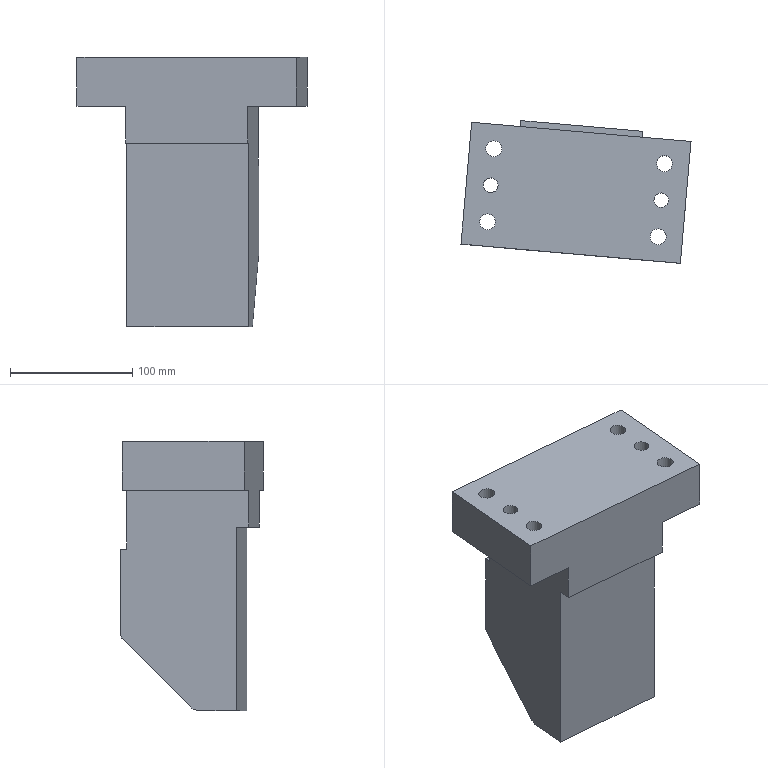Part | NX | features solid 2 | 1 solid | 33 faces | box 188.031 x 116.802 x 220 mm | volume 2209901 mm3 | plane 18 | cylinder 11 | spline 3 | cone 1 | commonest cylinder face diameters 13 x4 20 x4 12 x3
STEP:
#1=CARTESIAN_POINT('',(273.786,-317.22,-120.));
#2=VERTEX_POINT('',#1);
#3=CARTESIAN_POINT('',(273.786,-311.22,-120.));
#4=DIRECTION('',(0.,0.,1.));
#5=DIRECTION('',(0.,-1.,0.));
#6=AXIS2_PLACEMENT_3D('',#3,#4,#5);
#7=CIRCLE('',#6,6.);
#8=EDGE_CURVE('',#2,#2,#7,.T.);
#9=ORIENTED_EDGE('',*,*,#8,.T.);
#10=EDGE_LOOP('',(#9));
#11=FACE_BOUND('',#10,.T.);
#12=CARTESIAN_POINT('',(225.156,-294.888,-120.));
#13=VERTEX_POINT('',#12);
#14=CARTESIAN_POINT('',(222.466,-325.628,-120.));
#15=VERTEX_POINT('',#14);
#16=CARTESIAN_POINT('',(230.746,-230.99,-120.));
#17=DIRECTION('',(-0.08716,-0.9962,0.));
#18=VECTOR('',#17,1000.);
#19=LINE('',#16,#18);
#20=EDGE_CURVE('',#13,#15,#19,.T.);
#21=ORIENTED_EDGE('',*,*,#20,.F.);
#22=CARTESIAN_POINT('',(324.775,-303.603,-120.));
#23=VERTEX_POINT('',#22);
#24=CARTESIAN_POINT('',(225.156,-294.888,-120.));
#25=CARTESIAN_POINT('',(258.362,-297.793,-120.));
#26=CARTESIAN_POINT('',(291.569,-300.698,-120.));
#27=CARTESIAN_POINT('',(324.775,-303.603,-120.));
#28=B_SPLINE_CURVE_WITH_KNOTS('',3,(#24,#25,#26,#27),.UNSPECIFIED.,.F.,.F.,(4,4),(0.,0.1),.UNSPECIFIED.);
#29=EDGE_CURVE('',#13,#23,#28,.T.);
#30=ORIENTED_EDGE('',*,*,#29,.T.);
#31=CARTESIAN_POINT('',(322.086,-334.344,-120.));
#32=VERTEX_POINT('',#31);
#33=CARTESIAN_POINT('',(330.365,-239.705,-120.));
#34=DIRECTION('',(-0.08716,-0.9962,0.));
#35=VECTOR('',#34,1000.);
#36=LINE('',#33,#35);
#37=EDGE_CURVE('',#23,#32,#36,.T.);
#38=ORIENTED_EDGE('',*,*,#37,.T.);
#39=CARTESIAN_POINT('',(322.086,-334.344,-120.));
#40=DIRECTION('',(0.9962,-0.08716,0.));
#41=VECTOR('',#40,1000.);
#42=LINE('',#39,#41);
#43=EDGE_CURVE('',#15,#32,#42,.T.);
#44=ORIENTED_EDGE('',*,*,#43,.F.);
#45=EDGE_LOOP('',(#21,#30,#38,#44));
#46=FACE_BOUND('',#45,.T.);
#47=CARTESIAN_POINT('',(330.365,-239.705,-120.));
#48=DIRECTION('',(0.,0.,-1.));
#49=DIRECTION('',(0.,1.,0.));
#50=AXIS2_PLACEMENT_3D('',#47,#48,#49);
#51=PLANE('',#50);
#52=ADVANCED_FACE('',(#11,#46),#51,.T.);
#53=CARTESIAN_POINT('',(230.618,-232.449,-61.464));
#54=VERTEX_POINT('',#53);
#55=CARTESIAN_POINT('',(225.772,-287.844,-117.071));
#56=VERTEX_POINT('',#55);
#57=CARTESIAN_POINT('',(228.872,-252.408,-81.5));
#58=DIRECTION('',(-0.06163,-0.7044,-0.7071));
#59=VECTOR('',#58,1000.);
#60=LINE('',#57,#59);
#61=EDGE_CURVE('',#54,#56,#60,.T.);
#62=ORIENTED_EDGE('',*,*,#61,.T.);
#63=CARTESIAN_POINT('',(225.156,-294.888,-110.));
#64=DIRECTION('',(-0.9962,0.08716,0.));
#65=DIRECTION('',(-0.08716,-0.9962,0.));
#66=AXIS2_PLACEMENT_3D('',#63,#64,#65);
#67=CIRCLE('',#66,10.);
#68=EDGE_CURVE('',#56,#13,#67,.T.);
#69=ORIENTED_EDGE('',*,*,#68,.T.);
#70=ORIENTED_EDGE('',*,*,#20,.T.);
#71=CARTESIAN_POINT('',(222.466,-325.628,30.));
#72=VERTEX_POINT('',#71);
#73=CARTESIAN_POINT('',(222.466,-325.628,-170.));
#74=DIRECTION('',(0.,0.,1.));
#75=VECTOR('',#74,1000.);
#76=LINE('',#73,#75);
#77=EDGE_CURVE('',#72,#15,#76,.F.);
#78=ORIENTED_EDGE('',*,*,#77,.F.);
#79=CARTESIAN_POINT('',(221.595,-335.59,30.));
#80=VERTEX_POINT('',#79);
#81=CARTESIAN_POINT('',(220.723,-345.552,30.));
#82=DIRECTION('',(-0.08716,-0.9962,0.));
#83=VECTOR('',#82,1000.);
#84=LINE('',#81,#83);
#85=EDGE_CURVE('',#80,#72,#84,.F.);
#86=ORIENTED_EDGE('',*,*,#85,.F.);
#87=CARTESIAN_POINT('',(221.595,-335.59,60.));
#88=VERTEX_POINT('',#87);
#89=CARTESIAN_POINT('',(221.595,-335.59,-103.));
#90=DIRECTION('',(0.,0.,1.));
#91=VECTOR('',#90,1000.);
#92=LINE('',#89,#91);
#93=EDGE_CURVE('',#80,#88,#92,.T.);
#94=ORIENTED_EDGE('',*,*,#93,.T.);
#95=CARTESIAN_POINT('',(230.31,-235.971,60.));
#96=VERTEX_POINT('',#95);
#97=CARTESIAN_POINT('',(212.443,-440.191,60.));
#98=DIRECTION('',(0.08716,0.9962,0.));
#99=VECTOR('',#98,1000.);
#100=LINE('',#97,#99);
#101=EDGE_CURVE('',#88,#96,#100,.T.);
#102=ORIENTED_EDGE('',*,*,#101,.T.);
#103=CARTESIAN_POINT('',(230.31,-235.971,12.));
#104=VERTEX_POINT('',#103);
#105=CARTESIAN_POINT('',(230.31,-235.971,57.));
#106=DIRECTION('',(0.,0.,-1.));
#107=VECTOR('',#106,1000.);
#108=LINE('',#105,#107);
#109=EDGE_CURVE('',#96,#104,#108,.T.);
#110=ORIENTED_EDGE('',*,*,#109,.T.);
#111=CARTESIAN_POINT('',(230.746,-230.99,12.));
#112=VERTEX_POINT('',#111);
#113=CARTESIAN_POINT('',(230.746,-230.99,12.));
#114=DIRECTION('',(0.08716,0.9962,0.));
#115=VECTOR('',#114,1000.);
#116=LINE('',#113,#115);
#117=EDGE_CURVE('',#104,#112,#116,.T.);
#118=ORIENTED_EDGE('',*,*,#117,.T.);
#119=CARTESIAN_POINT('',(230.746,-230.99,-57.929));
#120=VERTEX_POINT('',#119);
#121=CARTESIAN_POINT('',(230.746,-230.99,-103.));
#122=DIRECTION('',(0.,0.,1.));
#123=VECTOR('',#122,1000.);
#124=LINE('',#121,#123);
#125=EDGE_CURVE('',#112,#120,#124,.F.);
#126=ORIENTED_EDGE('',*,*,#125,.T.);
#127=CARTESIAN_POINT('',(230.31,-235.971,-57.929));
#128=DIRECTION('',(-0.9962,0.08716,0.));
#129=DIRECTION('',(-0.08716,-0.9962,0.));
#130=AXIS2_PLACEMENT_3D('',#127,#128,#129);
#131=CIRCLE('',#130,5.);
#132=EDGE_CURVE('',#120,#54,#131,.T.);
#133=ORIENTED_EDGE('',*,*,#132,.T.);
#134=EDGE_LOOP('',(#62,#69,#70,#78,#86,#94,#102,#110,#118,#126,#133));
#135=FACE_BOUND('',#134,.T.);
#136=CARTESIAN_POINT('',(230.746,-230.99,-103.));
#137=DIRECTION('',(-0.9962,0.08716,0.));
#138=DIRECTION('',(0.,0.,1.));
#139=AXIS2_PLACEMENT_3D('',#136,#137,#138);
#140=PLANE('',#139);
#141=ADVANCED_FACE('',(#135),#140,.T.);
#142=ORIENTED_EDGE('',*,*,#37,.F.);
#143=CARTESIAN_POINT('',(325.391,-296.559,-117.071));
#144=VERTEX_POINT('',#143);
#145=CARTESIAN_POINT('',(324.775,-303.603,-110.));
#146=DIRECTION('',(-0.9962,0.08716,0.));
#147=DIRECTION('',(-0.08716,-0.9962,0.));
#148=AXIS2_PLACEMENT_3D('',#145,#146,#147);
#149=CIRCLE('',#148,10.);
#150=EDGE_CURVE('',#23,#144,#149,.F.);
#151=ORIENTED_EDGE('',*,*,#150,.T.);
#152=CARTESIAN_POINT('',(330.238,-241.164,-61.464));
#153=VERTEX_POINT('',#152);
#154=CARTESIAN_POINT('',(328.492,-261.124,-81.5));
#155=DIRECTION('',(-0.06163,-0.7044,-0.7071));
#156=VECTOR('',#155,1000.);
#157=LINE('',#154,#156);
#158=EDGE_CURVE('',#153,#144,#157,.T.);
#159=ORIENTED_EDGE('',*,*,#158,.F.);
#160=CARTESIAN_POINT('',(330.365,-239.705,-57.929));
#161=VERTEX_POINT('',#160);
#162=CARTESIAN_POINT('',(329.93,-244.686,-57.929));
#163=DIRECTION('',(-0.9962,0.08716,0.));
#164=DIRECTION('',(-0.08716,-0.9962,0.));
#165=AXIS2_PLACEMENT_3D('',#162,#163,#164);
#166=CIRCLE('',#165,5.);
#167=EDGE_CURVE('',#153,#161,#166,.F.);
#168=ORIENTED_EDGE('',*,*,#167,.T.);
#169=CARTESIAN_POINT('',(330.365,-239.705,12.));
#170=VERTEX_POINT('',#169);
#171=CARTESIAN_POINT('',(330.365,-239.705,-103.));
#172=DIRECTION('',(0.,0.,1.));
#173=VECTOR('',#172,1000.);
#174=LINE('',#171,#173);
#175=EDGE_CURVE('',#170,#161,#174,.F.);
#176=ORIENTED_EDGE('',*,*,#175,.F.);
#177=CARTESIAN_POINT('',(329.93,-244.686,12.));
#178=VERTEX_POINT('',#177);
#179=CARTESIAN_POINT('',(330.365,-239.705,12.));
#180=DIRECTION('',(0.08716,0.9962,0.));
#181=VECTOR('',#180,1000.);
#182=LINE('',#179,#181);
#183=EDGE_CURVE('',#178,#170,#182,.T.);
#184=ORIENTED_EDGE('',*,*,#183,.F.);
#185=CARTESIAN_POINT('',(329.93,-244.686,60.));
#186=VERTEX_POINT('',#185);
#187=CARTESIAN_POINT('',(329.93,-244.686,57.));
#188=DIRECTION('',(0.,0.,-1.));
#189=VECTOR('',#188,1000.);
#190=LINE('',#187,#189);
#191=EDGE_CURVE('',#186,#178,#190,.T.);
#192=ORIENTED_EDGE('',*,*,#191,.F.);
#193=CARTESIAN_POINT('',(321.214,-344.306,60.));
#194=VERTEX_POINT('',#193);
#195=CARTESIAN_POINT('',(312.063,-448.906,60.));
#196=DIRECTION('',(0.08716,0.9962,0.));
#197=VECTOR('',#196,1000.);
#198=LINE('',#195,#197);
#199=EDGE_CURVE('',#194,#186,#198,.T.);
#200=ORIENTED_EDGE('',*,*,#199,.F.);
#201=CARTESIAN_POINT('',(321.214,-344.306,30.));
#202=VERTEX_POINT('',#201);
#203=CARTESIAN_POINT('',(321.214,-344.306,-103.));
#204=DIRECTION('',(0.,0.,1.));
#205=VECTOR('',#204,1000.);
#206=LINE('',#203,#205);
#207=EDGE_CURVE('',#202,#194,#206,.T.);
#208=ORIENTED_EDGE('',*,*,#207,.F.);
#209=CARTESIAN_POINT('',(322.086,-334.344,30.));
#210=VERTEX_POINT('',#209);
#211=CARTESIAN_POINT('',(320.343,-354.268,30.));
#212=DIRECTION('',(-0.08716,-0.9962,0.));
#213=VECTOR('',#212,1000.);
#214=LINE('',#211,#213);
#215=EDGE_CURVE('',#202,#210,#214,.F.);
#216=ORIENTED_EDGE('',*,*,#215,.T.);
#217=CARTESIAN_POINT('',(322.086,-334.344,-170.));
#218=DIRECTION('',(0.,0.,-1.));
#219=VECTOR('',#218,1000.);
#220=LINE('',#217,#219);
#221=EDGE_CURVE('',#32,#210,#220,.F.);
#222=ORIENTED_EDGE('',*,*,#221,.F.);
#223=EDGE_LOOP('',(#142,#151,#159,#168,#176,#184,#192,#200,#208,#216,#222));
#224=FACE_BOUND('',#223,.T.);
#225=CARTESIAN_POINT('',(330.365,-239.705,-103.));
#226=DIRECTION('',(-0.9962,0.08716,0.));
#227=DIRECTION('',(0.,0.,1.));
#228=AXIS2_PLACEMENT_3D('',#225,#226,#227);
#229=PLANE('',#228);
#230=ADVANCED_FACE('',(#224),#229,.F.);
#231=ORIENTED_EDGE('',*,*,#175,.T.);
#232=CARTESIAN_POINT('',(330.365,-239.705,-57.929));
#233=CARTESIAN_POINT('',(297.159,-236.8,-57.929));
#234=CARTESIAN_POINT('',(263.952,-233.895,-57.929));
#235=CARTESIAN_POINT('',(230.746,-230.99,-57.929));
#236=B_SPLINE_CURVE_WITH_KNOTS('',3,(#232,#233,#234,#235),.UNSPECIFIED.,.F.,.F.,(4,4),(0.,0.1),.UNSPECIFIED.);
#237=EDGE_CURVE('',#161,#120,#236,.T.);
#238=ORIENTED_EDGE('',*,*,#237,.T.);
#239=ORIENTED_EDGE('',*,*,#125,.F.);
#240=CARTESIAN_POINT('',(330.365,-239.705,12.));
#241=DIRECTION('',(0.9962,-0.08716,0.));
#242=VECTOR('',#241,1000.);
#243=LINE('',#240,#242);
#244=EDGE_CURVE('',#170,#112,#243,.F.);
#245=ORIENTED_EDGE('',*,*,#244,.F.);
#246=EDGE_LOOP('',(#231,#238,#239,#245));
#247=FACE_BOUND('',#246,.T.);
#248=CARTESIAN_POINT('',(330.365,-239.705,-80.));
#249=DIRECTION('',(-0.08716,-0.9962,0.));
#250=DIRECTION('',(0.9962,-0.08716,0.));
#251=AXIS2_PLACEMENT_3D('',#248,#249,#250);
#252=PLANE('',#251);
#253=ADVANCED_FACE('',(#247),#252,.F.);
#254=ORIENTED_EDGE('',*,*,#93,.F.);
#255=CARTESIAN_POINT('',(321.214,-344.306,30.));
#256=DIRECTION('',(-0.9962,0.08716,0.));
#257=VECTOR('',#256,1000.);
#258=LINE('',#255,#257);
#259=EDGE_CURVE('',#80,#202,#258,.F.);
#260=ORIENTED_EDGE('',*,*,#259,.T.);
#261=ORIENTED_EDGE('',*,*,#207,.T.);
#262=CARTESIAN_POINT('',(361.062,-347.792,60.));
#263=VERTEX_POINT('',#262);
#264=CARTESIAN_POINT('',(321.214,-344.306,60.));
#265=DIRECTION('',(-0.9962,0.08716,0.));
#266=VECTOR('',#265,1000.);
#267=LINE('',#264,#266);
#268=EDGE_CURVE('',#263,#194,#267,.T.);
#269=ORIENTED_EDGE('',*,*,#268,.F.);
#270=CARTESIAN_POINT('',(361.062,-347.792,100.));
#271=VERTEX_POINT('',#270);
#272=CARTESIAN_POINT('',(361.062,-347.792,102.));
#273=DIRECTION('',(0.,0.,-1.));
#274=VECTOR('',#273,1000.);
#275=LINE('',#272,#274);
#276=EDGE_CURVE('',#271,#263,#275,.T.);
#277=ORIENTED_EDGE('',*,*,#276,.F.);
#278=CARTESIAN_POINT('',(181.747,-332.104,100.));
#279=VERTEX_POINT('',#278);
#280=CARTESIAN_POINT('',(321.214,-344.306,100.));
#281=DIRECTION('',(-0.9962,0.08716,0.));
#282=VECTOR('',#281,1000.);
#283=LINE('',#280,#282);
#284=EDGE_CURVE('',#271,#279,#283,.T.);
#285=ORIENTED_EDGE('',*,*,#284,.T.);
#286=CARTESIAN_POINT('',(181.747,-332.104,60.));
#287=VERTEX_POINT('',#286);
#288=CARTESIAN_POINT('',(181.747,-332.104,-103.));
#289=DIRECTION('',(0.,0.,-1.));
#290=VECTOR('',#289,1000.);
#291=LINE('',#288,#290);
#292=EDGE_CURVE('',#279,#287,#291,.T.);
#293=ORIENTED_EDGE('',*,*,#292,.T.);
#294=CARTESIAN_POINT('',(108.527,-325.698,60.));
#295=DIRECTION('',(0.9962,-0.08716,0.));
#296=VECTOR('',#295,1000.);
#297=LINE('',#294,#296);
#298=EDGE_CURVE('',#287,#88,#297,.T.);
#299=ORIENTED_EDGE('',*,*,#298,.T.);
#300=EDGE_LOOP('',(#254,#260,#261,#269,#277,#285,#293,#299));
#301=FACE_BOUND('',#300,.T.);
#302=CARTESIAN_POINT('',(321.214,-344.306,-103.));
#303=DIRECTION('',(-0.08716,-0.9962,0.));
#304=DIRECTION('',(0.,0.,-1.));
#305=AXIS2_PLACEMENT_3D('',#302,#303,#304);
#306=PLANE('',#305);
#307=ADVANCED_FACE('',(#301),#306,.T.);
#308=CARTESIAN_POINT('',(329.93,-244.686,12.));
#309=DIRECTION('',(-0.9962,0.08716,0.));
#310=VECTOR('',#309,1000.);
#311=LINE('',#308,#310);
#312=EDGE_CURVE('',#178,#104,#311,.T.);
#313=ORIENTED_EDGE('',*,*,#312,.F.);
#314=ORIENTED_EDGE('',*,*,#183,.T.);
#315=ORIENTED_EDGE('',*,*,#244,.T.);
#316=ORIENTED_EDGE('',*,*,#117,.F.);
#317=EDGE_LOOP('',(#313,#314,#315,#316));
#318=FACE_BOUND('',#317,.T.);
#319=CARTESIAN_POINT('',(327.751,-269.591,12.));
#320=DIRECTION('',(0.,0.,1.));
#321=DIRECTION('',(0.,-1.,0.));
#322=AXIS2_PLACEMENT_3D('',#319,#320,#321);
#323=PLANE('',#322);
#324=ADVANCED_FACE('',(#318),#323,.T.);
#325=ORIENTED_EDGE('',*,*,#312,.T.);
#326=ORIENTED_EDGE('',*,*,#109,.F.);
#327=CARTESIAN_POINT('',(190.462,-232.485,60.));
#328=VERTEX_POINT('',#327);
#329=CARTESIAN_POINT('',(117.242,-226.079,60.));
#330=DIRECTION('',(0.9962,-0.08716,0.));
#331=VECTOR('',#330,1000.);
#332=LINE('',#329,#331);
#333=EDGE_CURVE('',#328,#96,#332,.T.);
#334=ORIENTED_EDGE('',*,*,#333,.F.);
#335=CARTESIAN_POINT('',(190.462,-232.485,100.));
#336=VERTEX_POINT('',#335);
#337=CARTESIAN_POINT('',(190.462,-232.485,57.));
#338=DIRECTION('',(0.,0.,-1.));
#339=VECTOR('',#338,1000.);
#340=LINE('',#337,#339);
#341=EDGE_CURVE('',#336,#328,#340,.T.);
#342=ORIENTED_EDGE('',*,*,#341,.F.);
#343=CARTESIAN_POINT('',(369.777,-248.173,100.));
#344=VERTEX_POINT('',#343);
#345=CARTESIAN_POINT('',(329.93,-244.686,100.));
#346=DIRECTION('',(-0.9962,0.08716,0.));
#347=VECTOR('',#346,1000.);
#348=LINE('',#345,#347);
#349=EDGE_CURVE('',#344,#336,#348,.T.);
#350=ORIENTED_EDGE('',*,*,#349,.F.);
#351=CARTESIAN_POINT('',(369.777,-248.173,60.));
#352=VERTEX_POINT('',#351);
#353=CARTESIAN_POINT('',(369.777,-248.173,102.));
#354=DIRECTION('',(0.,0.,-1.));
#355=VECTOR('',#354,1000.);
#356=LINE('',#353,#355);
#357=EDGE_CURVE('',#344,#352,#356,.T.);
#358=ORIENTED_EDGE('',*,*,#357,.T.);
#359=CARTESIAN_POINT('',(267.667,-239.239,60.));
#360=DIRECTION('',(-0.9962,0.08716,0.));
#361=VECTOR('',#360,1000.);
#362=LINE('',#359,#361);
#363=EDGE_CURVE('',#352,#186,#362,.T.);
#364=ORIENTED_EDGE('',*,*,#363,.T.);
#365=ORIENTED_EDGE('',*,*,#191,.T.);
#366=EDGE_LOOP('',(#325,#326,#334,#342,#350,#358,#364,#365));
#367=FACE_BOUND('',#366,.T.);
#368=CARTESIAN_POINT('',(329.93,-244.686,57.));
#369=DIRECTION('',(-0.08716,-0.9962,0.));
#370=DIRECTION('',(0.9962,-0.08716,0.));
#371=AXIS2_PLACEMENT_3D('',#368,#369,#370);
#372=PLANE('',#371);
#373=ADVANCED_FACE('',(#367),#372,.F.);
#374=CARTESIAN_POINT('',(206.029,-290.037,100.));
#375=VERTEX_POINT('',#374);
#376=CARTESIAN_POINT('',(206.029,-284.037,100.));
#377=DIRECTION('',(0.,0.,1.));
#378=DIRECTION('',(0.,-1.,0.));
#379=AXIS2_PLACEMENT_3D('',#376,#377,#378);
#380=CIRCLE('',#379,6.);
#381=EDGE_CURVE('',#375,#375,#380,.T.);
#382=ORIENTED_EDGE('',*,*,#381,.F.);
#383=EDGE_LOOP('',(#382));
#384=FACE_BOUND('',#383,.T.);
#385=CARTESIAN_POINT('',(345.496,-302.239,100.));
#386=VERTEX_POINT('',#385);
#387=CARTESIAN_POINT('',(345.496,-296.239,100.));
#388=DIRECTION('',(0.,0.,1.));
#389=DIRECTION('',(0.,-1.,0.));
#390=AXIS2_PLACEMENT_3D('',#387,#388,#389);
#391=CIRCLE('',#390,6.);
#392=EDGE_CURVE('',#386,#386,#391,.T.);
#393=ORIENTED_EDGE('',*,*,#392,.F.);
#394=EDGE_LOOP('',(#393));
#395=FACE_BOUND('',#394,.T.);
#396=CARTESIAN_POINT('',(203.414,-320.423,100.));
#397=VERTEX_POINT('',#396);
#398=CARTESIAN_POINT('',(203.414,-313.923,100.));
#399=DIRECTION('',(0.,0.,1.));
#400=DIRECTION('',(0.,-1.,0.));
#401=AXIS2_PLACEMENT_3D('',#398,#399,#400);
#402=CIRCLE('',#401,6.5);
#403=EDGE_CURVE('',#397,#397,#402,.T.);
#404=ORIENTED_EDGE('',*,*,#403,.F.);
#405=EDGE_LOOP('',(#404));
#406=FACE_BOUND('',#405,.T.);
#407=CARTESIAN_POINT('',(208.643,-260.652,100.));
#408=VERTEX_POINT('',#407);
#409=CARTESIAN_POINT('',(208.643,-254.152,100.));
#410=DIRECTION('',(0.,0.,1.));
#411=DIRECTION('',(0.,-1.,0.));
#412=AXIS2_PLACEMENT_3D('',#409,#410,#411);
#413=CIRCLE('',#412,6.5);
#414=EDGE_CURVE('',#408,#408,#413,.T.);
#415=ORIENTED_EDGE('',*,*,#414,.F.);
#416=EDGE_LOOP('',(#415));
#417=FACE_BOUND('',#416,.T.);
#418=CARTESIAN_POINT('',(342.881,-332.625,100.));
#419=VERTEX_POINT('',#418);
#420=CARTESIAN_POINT('',(342.881,-326.125,100.));
#421=DIRECTION('',(0.,0.,1.));
#422=DIRECTION('',(0.,-1.,0.));
#423=AXIS2_PLACEMENT_3D('',#420,#421,#422);
#424=CIRCLE('',#423,6.5);
#425=EDGE_CURVE('',#419,#419,#424,.T.);
#426=ORIENTED_EDGE('',*,*,#425,.F.);
#427=EDGE_LOOP('',(#426));
#428=FACE_BOUND('',#427,.T.);
#429=CARTESIAN_POINT('',(348.11,-272.853,100.));
#430=VERTEX_POINT('',#429);
#431=CARTESIAN_POINT('',(348.11,-266.353,100.));
#432=DIRECTION('',(0.,0.,1.));
#433=DIRECTION('',(0.,-1.,0.));
#434=AXIS2_PLACEMENT_3D('',#431,#432,#433);
#435=CIRCLE('',#434,6.5);
#436=EDGE_CURVE('',#430,#430,#435,.T.);
#437=ORIENTED_EDGE('',*,*,#436,.F.);
#438=EDGE_LOOP('',(#437));
#439=FACE_BOUND('',#438,.T.);
#440=ORIENTED_EDGE('',*,*,#349,.T.);
#441=CARTESIAN_POINT('',(177.326,-382.632,100.));
#442=DIRECTION('',(0.08716,0.9962,0.));
#443=VECTOR('',#442,1000.);
#444=LINE('',#441,#443);
#445=EDGE_CURVE('',#279,#336,#444,.T.);
#446=ORIENTED_EDGE('',*,*,#445,.F.);
#447=ORIENTED_EDGE('',*,*,#284,.F.);
#448=CARTESIAN_POINT('',(367.599,-273.077,100.));
#449=DIRECTION('',(0.08716,0.9962,0.));
#450=VECTOR('',#449,1000.);
#451=LINE('',#448,#450);
#452=EDGE_CURVE('',#271,#344,#451,.T.);
#453=ORIENTED_EDGE('',*,*,#452,.T.);
#454=EDGE_LOOP('',(#440,#446,#447,#453));
#455=FACE_BOUND('',#454,.T.);
#456=CARTESIAN_POINT('',(327.751,-269.591,100.));
#457=DIRECTION('',(0.,0.,1.));
#458=DIRECTION('',(0.,-1.,0.));
#459=AXIS2_PLACEMENT_3D('',#456,#457,#458);
#460=PLANE('',#459);
#461=ADVANCED_FACE('',(#384,#395,#406,#417,#428,#439,#455),#460,.T.);
#462=ORIENTED_EDGE('',*,*,#85,.T.);
#463=CARTESIAN_POINT('',(192.58,-323.014,30.));
#464=DIRECTION('',(0.9962,-0.08716,0.));
#465=VECTOR('',#464,1000.);
#466=LINE('',#463,#465);
#467=EDGE_CURVE('',#210,#72,#466,.F.);
#468=ORIENTED_EDGE('',*,*,#467,.F.);
#469=ORIENTED_EDGE('',*,*,#215,.F.);
#470=ORIENTED_EDGE('',*,*,#259,.F.);
#471=EDGE_LOOP('',(#462,#468,#469,#470));
#472=FACE_BOUND('',#471,.T.);
#473=CARTESIAN_POINT('',(340.266,-356.011,30.));
#474=DIRECTION('',(0.,0.,1.));
#475=DIRECTION('',(0.9962,-0.08716,0.));
#476=AXIS2_PLACEMENT_3D('',#473,#474,#475);
#477=PLANE('',#476);
#478=ADVANCED_FACE('',(#472),#477,.F.);
#479=ORIENTED_EDGE('',*,*,#221,.T.);
#480=ORIENTED_EDGE('',*,*,#467,.T.);
#481=ORIENTED_EDGE('',*,*,#77,.T.);
#482=ORIENTED_EDGE('',*,*,#43,.T.);
#483=EDGE_LOOP('',(#479,#480,#481,#482));
#484=FACE_BOUND('',#483,.T.);
#485=CARTESIAN_POINT('',(192.58,-323.014,-170.));
#486=DIRECTION('',(0.08716,0.9962,0.));
#487=DIRECTION('',(0.,0.,-1.));
#488=AXIS2_PLACEMENT_3D('',#485,#486,#487);
#489=PLANE('',#488);
#490=ADVANCED_FACE('',(#484),#489,.F.);
#491=CARTESIAN_POINT('',(351.496,-296.239,60.));
#492=VERTEX_POINT('',#491);
#493=CARTESIAN_POINT('',(345.496,-296.239,60.));
#494=DIRECTION('',(0.,0.,1.));
#495=DIRECTION('',(1.,0.,0.));
#496=AXIS2_PLACEMENT_3D('',#493,#494,#495);
#497=CIRCLE('',#496,6.);
#498=EDGE_CURVE('',#492,#492,#497,.T.);
#499=ORIENTED_EDGE('',*,*,#498,.T.);
#500=EDGE_LOOP('',(#499));
#501=FACE_BOUND('',#500,.T.);
#502=CARTESIAN_POINT('',(352.881,-326.125,60.));
#503=VERTEX_POINT('',#502);
#504=CARTESIAN_POINT('',(342.881,-326.125,60.));
#505=DIRECTION('',(0.,0.,1.));
#506=DIRECTION('',(1.,0.,0.));
#507=AXIS2_PLACEMENT_3D('',#504,#505,#506);
#508=CIRCLE('',#507,10.);
#509=EDGE_CURVE('',#503,#503,#508,.T.);
#510=ORIENTED_EDGE('',*,*,#509,.T.);
#511=EDGE_LOOP('',(#510));
#512=FACE_BOUND('',#511,.T.);
#513=CARTESIAN_POINT('',(358.11,-266.353,60.));
#514=VERTEX_POINT('',#513);
#515=CARTESIAN_POINT('',(348.11,-266.353,60.));
#516=DIRECTION('',(0.,0.,1.));
#517=DIRECTION('',(1.,0.,0.));
#518=AXIS2_PLACEMENT_3D('',#515,#516,#517);
#519=CIRCLE('',#518,10.);
#520=EDGE_CURVE('',#514,#514,#519,.T.);
#521=ORIENTED_EDGE('',*,*,#520,.T.);
#522=EDGE_LOOP('',(#521));
#523=FACE_BOUND('',#522,.T.);
#524=CARTESIAN_POINT('',(351.911,-452.393,60.));
#525=DIRECTION('',(0.08716,0.9962,0.));
#526=VECTOR('',#525,1000.);
#527=LINE('',#524,#526);
#528=EDGE_CURVE('',#263,#352,#527,.T.);
#529=ORIENTED_EDGE('',*,*,#528,.F.);
#530=ORIENTED_EDGE('',*,*,#268,.T.);
#531=ORIENTED_EDGE('',*,*,#199,.T.);
#532=ORIENTED_EDGE('',*,*,#363,.F.);
#533=EDGE_LOOP('',(#529,#530,#531,#532));
#534=FACE_BOUND('',#533,.T.);
#535=CARTESIAN_POINT('',(459.998,-461.849,60.));
#536=DIRECTION('',(0.,0.,1.));
#537=DIRECTION('',(-0.08716,-0.9962,0.));
#538=AXIS2_PLACEMENT_3D('',#535,#536,#537);
#539=PLANE('',#538);
#540=ADVANCED_FACE('',(#501,#512,#523,#534),#539,.F.);
#541=ORIENTED_EDGE('',*,*,#528,.T.);
#542=ORIENTED_EDGE('',*,*,#357,.F.);
#543=ORIENTED_EDGE('',*,*,#452,.F.);
#544=ORIENTED_EDGE('',*,*,#276,.T.);
#545=EDGE_LOOP('',(#541,#542,#543,#544));
#546=FACE_BOUND('',#545,.T.);
#547=CARTESIAN_POINT('',(356.641,-398.32,102.));
#548=DIRECTION('',(0.9962,-0.08716,0.));
#549=DIRECTION('',(0.,0.,-1.));
#550=AXIS2_PLACEMENT_3D('',#547,#548,#549);
#551=PLANE('',#550);
#552=ADVANCED_FACE('',(#546),#551,.T.);
#553=CARTESIAN_POINT('',(212.029,-284.037,60.));
#554=VERTEX_POINT('',#553);
#555=CARTESIAN_POINT('',(206.029,-284.037,60.));
#556=DIRECTION('',(0.,0.,1.));
#557=DIRECTION('',(1.,0.,0.));
#558=AXIS2_PLACEMENT_3D('',#555,#556,#557);
#559=CIRCLE('',#558,6.);
#560=EDGE_CURVE('',#554,#554,#559,.T.);
#561=ORIENTED_EDGE('',*,*,#560,.T.);
#562=EDGE_LOOP('',(#561));
#563=FACE_BOUND('',#562,.T.);
#564=CARTESIAN_POINT('',(213.414,-313.923,60.));
#565=VERTEX_POINT('',#564);
#566=CARTESIAN_POINT('',(203.414,-313.923,60.));
#567=DIRECTION('',(0.,0.,1.));
#568=DIRECTION('',(1.,0.,0.));
#569=AXIS2_PLACEMENT_3D('',#566,#567,#568);
#570=CIRCLE('',#569,10.);
#571=EDGE_CURVE('',#565,#565,#570,.T.);
#572=ORIENTED_EDGE('',*,*,#571,.T.);
#573=EDGE_LOOP('',(#572));
#574=FACE_BOUND('',#573,.T.);
#575=CARTESIAN_POINT('',(218.643,-254.152,60.));
#576=VERTEX_POINT('',#575);
#577=CARTESIAN_POINT('',(208.643,-254.152,60.));
#578=DIRECTION('',(0.,0.,1.));
#579=DIRECTION('',(1.,0.,0.));
#580=AXIS2_PLACEMENT_3D('',#577,#578,#579);
#581=CIRCLE('',#580,10.);
#582=EDGE_CURVE('',#576,#576,#581,.T.);
#583=ORIENTED_EDGE('',*,*,#582,.T.);
#584=EDGE_LOOP('',(#583));
#585=FACE_BOUND('',#584,.T.);
#586=CARTESIAN_POINT('',(177.326,-382.632,60.));
#587=DIRECTION('',(0.08716,0.9962,0.));
#588=VECTOR('',#587,1000.);
#589=LINE('',#586,#588);
#590=EDGE_CURVE('',#287,#328,#589,.T.);
#591=ORIENTED_EDGE('',*,*,#590,.T.);
#592=ORIENTED_EDGE('',*,*,#333,.T.);
#593=ORIENTED_EDGE('',*,*,#101,.F.);
#594=ORIENTED_EDGE('',*,*,#298,.F.);
#595=EDGE_LOOP('',(#591,#592,#593,#594));
#596=FACE_BOUND('',#595,.T.);
#597=CARTESIAN_POINT('',(99.375,-430.299,60.));
#598=DIRECTION('',(0.,0.,1.));
#599=DIRECTION('',(-0.08716,-0.9962,0.));
#600=AXIS2_PLACEMENT_3D('',#597,#598,#599);
#601=PLANE('',#600);
#602=ADVANCED_FACE('',(#563,#574,#585,#596),#601,.F.);
#603=ORIENTED_EDGE('',*,*,#590,.F.);
#604=ORIENTED_EDGE('',*,*,#292,.F.);
#605=ORIENTED_EDGE('',*,*,#445,.T.);
#606=ORIENTED_EDGE('',*,*,#341,.T.);
#607=EDGE_LOOP('',(#603,#604,#605,#606));
#608=FACE_BOUND('',#607,.T.);
#609=CARTESIAN_POINT('',(177.326,-382.632,102.));
#610=DIRECTION('',(-0.9962,0.08716,0.));
#611=DIRECTION('',(0.,0.,-1.));
#612=AXIS2_PLACEMENT_3D('',#609,#610,#611);
#613=PLANE('',#612);
#614=ADVANCED_FACE('',(#608),#613,.T.);
#615=CARTESIAN_POINT('',(348.11,-256.353,75.));
#616=VERTEX_POINT('',#615);
#617=CARTESIAN_POINT('',(348.11,-266.353,75.));
#618=DIRECTION('',(0.,0.,-1.));
#619=DIRECTION('',(0.,1.,0.));
#620=AXIS2_PLACEMENT_3D('',#617,#618,#619);
#621=CIRCLE('',#620,10.);
#622=EDGE_CURVE('',#616,#616,#621,.T.);
#623=ORIENTED_EDGE('',*,*,#622,.F.);
#624=EDGE_LOOP('',(#623));
#625=FACE_BOUND('',#624,.T.);
#626=ORIENTED_EDGE('',*,*,#520,.F.);
#627=EDGE_LOOP('',(#626));
#628=FACE_BOUND('',#627,.T.);
#629=CARTESIAN_POINT('',(348.11,-266.353,75.));
#630=DIRECTION('',(0.,0.,-1.));
#631=DIRECTION('',(0.,1.,0.));
#632=AXIS2_PLACEMENT_3D('',#629,#630,#631);
#633=CYLINDRICAL_SURFACE('',#632,10.);
#634=ADVANCED_FACE('',(#625,#628),#633,.F.);
#635=ORIENTED_EDGE('',*,*,#436,.T.);
#636=EDGE_LOOP('',(#635));
#637=FACE_BOUND('',#636,.T.);
#638=CARTESIAN_POINT('',(348.11,-272.853,75.));
#639=VERTEX_POINT('',#638);
#640=CARTESIAN_POINT('',(348.11,-266.353,75.));
#641=DIRECTION('',(0.,0.,1.));
#642=DIRECTION('',(0.,-1.,0.));
#643=AXIS2_PLACEMENT_3D('',#640,#641,#642);
#644=CIRCLE('',#643,6.5);
#645=EDGE_CURVE('',#639,#639,#644,.F.);
#646=ORIENTED_EDGE('',*,*,#645,.T.);
#647=EDGE_LOOP('',(#646));
#648=FACE_BOUND('',#647,.T.);
#649=CARTESIAN_POINT('',(348.11,-266.353,125.));
#650=DIRECTION('',(0.,0.,-1.));
#651=DIRECTION('',(0.,1.,0.));
#652=AXIS2_PLACEMENT_3D('',#649,#650,#651);
#653=CYLINDRICAL_SURFACE('',#652,6.5);
#654=ADVANCED_FACE('',(#637,#648),#653,.F.);
#655=ORIENTED_EDGE('',*,*,#645,.F.);
#656=EDGE_LOOP('',(#655));
#657=FACE_BOUND('',#656,.T.);
#658=ORIENTED_EDGE('',*,*,#622,.T.);
#659=EDGE_LOOP('',(#658));
#660=FACE_BOUND('',#659,.T.);
#661=CARTESIAN_POINT('',(348.11,-266.353,75.));
#662=DIRECTION('',(0.,0.,1.));
#663=DIRECTION('',(0.,-1.,0.));
#664=AXIS2_PLACEMENT_3D('',#661,#662,#663);
#665=PLANE('',#664);
#666=ADVANCED_FACE('',(#657,#660),#665,.F.);
#667=CARTESIAN_POINT('',(342.881,-316.125,75.));
#668=VERTEX_POINT('',#667);
#669=CARTESIAN_POINT('',(342.881,-326.125,75.));
#670=DIRECTION('',(0.,0.,-1.));
#671=DIRECTION('',(0.,1.,0.));
#672=AXIS2_PLACEMENT_3D('',#669,#670,#671);
#673=CIRCLE('',#672,10.);
#674=EDGE_CURVE('',#668,#668,#673,.T.);
#675=ORIENTED_EDGE('',*,*,#674,.F.);
#676=EDGE_LOOP('',(#675));
#677=FACE_BOUND('',#676,.T.);
#678=ORIENTED_EDGE('',*,*,#509,.F.);
#679=EDGE_LOOP('',(#678));
#680=FACE_BOUND('',#679,.T.);
#681=CARTESIAN_POINT('',(342.881,-326.125,75.));
#682=DIRECTION('',(0.,0.,-1.));
#683=DIRECTION('',(0.,1.,0.));
#684=AXIS2_PLACEMENT_3D('',#681,#682,#683);
#685=CYLINDRICAL_SURFACE('',#684,10.);
#686=ADVANCED_FACE('',(#677,#680),#685,.F.);
#687=ORIENTED_EDGE('',*,*,#425,.T.);
#688=EDGE_LOOP('',(#687));
#689=FACE_BOUND('',#688,.T.);
#690=CARTESIAN_POINT('',(342.881,-332.625,75.));
#691=VERTEX_POINT('',#690);
#692=CARTESIAN_POINT('',(342.881,-326.125,75.));
#693=DIRECTION('',(0.,0.,1.));
#694=DIRECTION('',(0.,-1.,0.));
#695=AXIS2_PLACEMENT_3D('',#692,#693,#694);
#696=CIRCLE('',#695,6.5);
#697=EDGE_CURVE('',#691,#691,#696,.F.);
#698=ORIENTED_EDGE('',*,*,#697,.T.);
#699=EDGE_LOOP('',(#698));
#700=FACE_BOUND('',#699,.T.);
#701=CARTESIAN_POINT('',(342.881,-326.125,125.));
#702=DIRECTION('',(0.,0.,-1.));
#703=DIRECTION('',(0.,1.,0.));
#704=AXIS2_PLACEMENT_3D('',#701,#702,#703);
#705=CYLINDRICAL_SURFACE('',#704,6.5);
#706=ADVANCED_FACE('',(#689,#700),#705,.F.);
#707=ORIENTED_EDGE('',*,*,#697,.F.);
#708=EDGE_LOOP('',(#707));
#709=FACE_BOUND('',#708,.T.);
#710=ORIENTED_EDGE('',*,*,#674,.T.);
#711=EDGE_LOOP('',(#710));
#712=FACE_BOUND('',#711,.T.);
#713=CARTESIAN_POINT('',(342.881,-326.125,75.));
#714=DIRECTION('',(0.,0.,1.));
#715=DIRECTION('',(0.,-1.,0.));
#716=AXIS2_PLACEMENT_3D('',#713,#714,#715);
#717=PLANE('',#716);
#718=ADVANCED_FACE('',(#709,#712),#717,.F.);
#719=CARTESIAN_POINT('',(208.643,-244.152,75.));
#720=VERTEX_POINT('',#719);
#721=CARTESIAN_POINT('',(208.643,-254.152,75.));
#722=DIRECTION('',(0.,0.,-1.));
#723=DIRECTION('',(0.,1.,0.));
#724=AXIS2_PLACEMENT_3D('',#721,#722,#723);
#725=CIRCLE('',#724,10.);
#726=EDGE_CURVE('',#720,#720,#725,.T.);
#727=ORIENTED_EDGE('',*,*,#726,.F.);
#728=EDGE_LOOP('',(#727));
#729=FACE_BOUND('',#728,.T.);
#730=ORIENTED_EDGE('',*,*,#582,.F.);
#731=EDGE_LOOP('',(#730));
#732=FACE_BOUND('',#731,.T.);
#733=CARTESIAN_POINT('',(208.643,-254.152,75.));
#734=DIRECTION('',(0.,0.,-1.));
#735=DIRECTION('',(0.,1.,0.));
#736=AXIS2_PLACEMENT_3D('',#733,#734,#735);
#737=CYLINDRICAL_SURFACE('',#736,10.);
#738=ADVANCED_FACE('',(#729,#732),#737,.F.);
#739=ORIENTED_EDGE('',*,*,#414,.T.);
#740=EDGE_LOOP('',(#739));
#741=FACE_BOUND('',#740,.T.);
#742=CARTESIAN_POINT('',(208.643,-260.652,75.));
#743=VERTEX_POINT('',#742);
#744=CARTESIAN_POINT('',(208.643,-254.152,75.));
#745=DIRECTION('',(0.,0.,1.));
#746=DIRECTION('',(0.,-1.,0.));
#747=AXIS2_PLACEMENT_3D('',#744,#745,#746);
#748=CIRCLE('',#747,6.5);
#749=EDGE_CURVE('',#743,#743,#748,.F.);
#750=ORIENTED_EDGE('',*,*,#749,.T.);
#751=EDGE_LOOP('',(#750));
#752=FACE_BOUND('',#751,.T.);
#753=CARTESIAN_POINT('',(208.643,-254.152,125.));
#754=DIRECTION('',(0.,0.,-1.));
#755=DIRECTION('',(0.,1.,0.));
#756=AXIS2_PLACEMENT_3D('',#753,#754,#755);
#757=CYLINDRICAL_SURFACE('',#756,6.5);
#758=ADVANCED_FACE('',(#741,#752),#757,.F.);
#759=ORIENTED_EDGE('',*,*,#749,.F.);
#760=EDGE_LOOP('',(#759));
#761=FACE_BOUND('',#760,.T.);
#762=ORIENTED_EDGE('',*,*,#726,.T.);
#763=EDGE_LOOP('',(#762));
#764=FACE_BOUND('',#763,.T.);
#765=CARTESIAN_POINT('',(208.643,-254.152,75.));
#766=DIRECTION('',(0.,0.,1.));
#767=DIRECTION('',(0.,-1.,0.));
#768=AXIS2_PLACEMENT_3D('',#765,#766,#767);
#769=PLANE('',#768);
#770=ADVANCED_FACE('',(#761,#764),#769,.F.);
#771=CARTESIAN_POINT('',(203.414,-303.923,75.));
#772=VERTEX_POINT('',#771);
#773=CARTESIAN_POINT('',(203.414,-313.923,75.));
#774=DIRECTION('',(0.,0.,-1.));
#775=DIRECTION('',(0.,1.,0.));
#776=AXIS2_PLACEMENT_3D('',#773,#774,#775);
#777=CIRCLE('',#776,10.);
#778=EDGE_CURVE('',#772,#772,#777,.T.);
#779=ORIENTED_EDGE('',*,*,#778,.F.);
#780=EDGE_LOOP('',(#779));
#781=FACE_BOUND('',#780,.T.);
#782=ORIENTED_EDGE('',*,*,#571,.F.);
#783=EDGE_LOOP('',(#782));
#784=FACE_BOUND('',#783,.T.);
#785=CARTESIAN_POINT('',(203.414,-313.923,75.));
#786=DIRECTION('',(0.,0.,-1.));
#787=DIRECTION('',(0.,1.,0.));
#788=AXIS2_PLACEMENT_3D('',#785,#786,#787);
#789=CYLINDRICAL_SURFACE('',#788,10.);
#790=ADVANCED_FACE('',(#781,#784),#789,.F.);
#791=ORIENTED_EDGE('',*,*,#403,.T.);
#792=EDGE_LOOP('',(#791));
#793=FACE_BOUND('',#792,.T.);
#794=CARTESIAN_POINT('',(203.414,-320.423,75.));
#795=VERTEX_POINT('',#794);
#796=CARTESIAN_POINT('',(203.414,-313.923,75.));
#797=DIRECTION('',(0.,0.,1.));
#798=DIRECTION('',(0.,-1.,0.));
#799=AXIS2_PLACEMENT_3D('',#796,#797,#798);
#800=CIRCLE('',#799,6.5);
#801=EDGE_CURVE('',#795,#795,#800,.F.);
#802=ORIENTED_EDGE('',*,*,#801,.T.);
#803=EDGE_LOOP('',(#802));
#804=FACE_BOUND('',#803,.T.);
#805=CARTESIAN_POINT('',(203.414,-313.923,125.));
#806=DIRECTION('',(0.,0.,-1.));
#807=DIRECTION('',(0.,1.,0.));
#808=AXIS2_PLACEMENT_3D('',#805,#806,#807);
#809=CYLINDRICAL_SURFACE('',#808,6.5);
#810=ADVANCED_FACE('',(#793,#804),#809,.F.);
#811=ORIENTED_EDGE('',*,*,#801,.F.);
#812=EDGE_LOOP('',(#811));
#813=FACE_BOUND('',#812,.T.);
#814=ORIENTED_EDGE('',*,*,#778,.T.);
#815=EDGE_LOOP('',(#814));
#816=FACE_BOUND('',#815,.T.);
#817=CARTESIAN_POINT('',(203.414,-313.923,75.));
#818=DIRECTION('',(0.,0.,1.));
#819=DIRECTION('',(0.,-1.,0.));
#820=AXIS2_PLACEMENT_3D('',#817,#818,#819);
#821=PLANE('',#820);
#822=ADVANCED_FACE('',(#813,#816),#821,.F.);
#823=ORIENTED_EDGE('',*,*,#392,.T.);
#824=EDGE_LOOP('',(#823));
#825=FACE_BOUND('',#824,.T.);
#826=ORIENTED_EDGE('',*,*,#498,.F.);
#827=EDGE_LOOP('',(#826));
#828=FACE_BOUND('',#827,.T.);
#829=CARTESIAN_POINT('',(345.496,-296.239,-25.));
#830=DIRECTION('',(0.,0.,1.));
#831=DIRECTION('',(1.,0.,0.));
#832=AXIS2_PLACEMENT_3D('',#829,#830,#831);
#833=CYLINDRICAL_SURFACE('',#832,6.);
#834=ADVANCED_FACE('',(#825,#828),#833,.F.);
#835=ORIENTED_EDGE('',*,*,#381,.T.);
#836=EDGE_LOOP('',(#835));
#837=FACE_BOUND('',#836,.T.);
#838=ORIENTED_EDGE('',*,*,#560,.F.);
#839=EDGE_LOOP('',(#838));
#840=FACE_BOUND('',#839,.T.);
#841=CARTESIAN_POINT('',(206.029,-284.037,-25.));
#842=DIRECTION('',(0.,0.,1.));
#843=DIRECTION('',(1.,0.,0.));
#844=AXIS2_PLACEMENT_3D('',#841,#842,#843);
#845=CYLINDRICAL_SURFACE('',#844,6.);
#846=ADVANCED_FACE('',(#837,#840),#845,.F.);
#847=ORIENTED_EDGE('',*,*,#158,.T.);
#848=CARTESIAN_POINT('',(325.391,-296.559,-117.071));
#849=CARTESIAN_POINT('',(292.185,-293.654,-117.071));
#850=CARTESIAN_POINT('',(258.978,-290.749,-117.071));
#851=CARTESIAN_POINT('',(225.772,-287.844,-117.071));
#852=B_SPLINE_CURVE_WITH_KNOTS('',3,(#848,#849,#850,#851),.UNSPECIFIED.,.F.,.F.,(4,4),(0.,0.1),.UNSPECIFIED.);
#853=EDGE_CURVE('',#144,#56,#852,.T.);
#854=ORIENTED_EDGE('',*,*,#853,.T.);
#855=ORIENTED_EDGE('',*,*,#61,.F.);
#856=CARTESIAN_POINT('',(230.618,-232.449,-61.464));
#857=CARTESIAN_POINT('',(263.825,-235.354,-61.464));
#858=CARTESIAN_POINT('',(297.031,-238.259,-61.464));
#859=CARTESIAN_POINT('',(330.238,-241.164,-61.464));
#860=B_SPLINE_CURVE_WITH_KNOTS('',3,(#856,#857,#858,#859),.UNSPECIFIED.,.F.,.F.,(4,4),(0.,0.1),.UNSPECIFIED.);
#861=EDGE_CURVE('',#54,#153,#860,.T.);
#862=ORIENTED_EDGE('',*,*,#861,.T.);
#863=EDGE_LOOP('',(#847,#854,#855,#862));
#864=FACE_BOUND('',#863,.T.);
#865=CARTESIAN_POINT('',(225.772,-287.844,-117.071));
#866=CARTESIAN_POINT('',(325.391,-296.559,-117.071));
#867=CARTESIAN_POINT('',(230.618,-232.449,-61.464));
#868=CARTESIAN_POINT('',(330.238,-241.164,-61.464));
#869=B_SPLINE_SURFACE_WITH_KNOTS('',1,1,((#865,#866),(#867,#868)),.PLANE_SURF.,.F.,.F.,.F.,(2,2),(2,2),(0.1712,0.5912),(0.3333,0.6667),.PIECEWISE_BEZIER_KNOTS.);
#870=ADVANCED_FACE('',(#864),#869,.T.);
#871=ORIENTED_EDGE('',*,*,#167,.F.);
#872=ORIENTED_EDGE('',*,*,#861,.F.);
#873=ORIENTED_EDGE('',*,*,#132,.F.);
#874=ORIENTED_EDGE('',*,*,#237,.F.);
#875=EDGE_LOOP('',(#871,#872,#873,#874));
#876=FACE_BOUND('',#875,.T.);
#877=CARTESIAN_POINT('',(330.238,-241.164,-61.464));
#878=CARTESIAN_POINT('',(330.365,-239.705,-60.));
#879=CARTESIAN_POINT('',(330.365,-239.705,-57.929));
#880=CARTESIAN_POINT('',(297.031,-238.259,-61.464));
#881=CARTESIAN_POINT('',(297.159,-236.8,-60.));
#882=CARTESIAN_POINT('',(297.159,-236.8,-57.929));
#883=CARTESIAN_POINT('',(263.825,-235.354,-61.464));
#884=CARTESIAN_POINT('',(263.952,-233.895,-60.));
#885=CARTESIAN_POINT('',(263.952,-233.895,-57.929));
#886=CARTESIAN_POINT('',(230.618,-232.449,-61.464));
#887=CARTESIAN_POINT('',(230.746,-230.99,-60.));
#888=CARTESIAN_POINT('',(230.746,-230.99,-57.929));
#889=(BOUNDED_SURFACE()B_SPLINE_SURFACE(3,2,((#877,#878,#879),(#880,#881,#882),(#883,#884,#885),(#886,#887,#888)),.UNSPECIFIED.,.F.,.F.,.F.)B_SPLINE_SURFACE_WITH_KNOTS((4,4),(3,3),(0.1373,0.2373),(0.,1.),.PIECEWISE_BEZIER_KNOTS.)GEOMETRIC_REPRESENTATION_ITEM()RATIONAL_B_SPLINE_SURFACE(((1.,0.9239,1.),(1.,0.9239,1.),(1.,0.9239,1.),(1.,0.9239,1.)))REPRESENTATION_ITEM('')SURFACE());
#890=ADVANCED_FACE('',(#876),#889,.T.);
#891=ORIENTED_EDGE('',*,*,#68,.F.);
#892=ORIENTED_EDGE('',*,*,#853,.F.);
#893=ORIENTED_EDGE('',*,*,#150,.F.);
#894=ORIENTED_EDGE('',*,*,#29,.F.);
#895=EDGE_LOOP('',(#891,#892,#893,#894));
#896=FACE_BOUND('',#895,.T.);
#897=CARTESIAN_POINT('',(225.772,-287.844,-117.071));
#898=CARTESIAN_POINT('',(225.517,-290.762,-120.));
#899=CARTESIAN_POINT('',(225.156,-294.888,-120.));
#900=CARTESIAN_POINT('',(258.978,-290.749,-117.071));
#901=CARTESIAN_POINT('',(258.723,-293.667,-120.));
#902=CARTESIAN_POINT('',(258.362,-297.793,-120.));
#903=CARTESIAN_POINT('',(292.185,-293.654,-117.071));
#904=CARTESIAN_POINT('',(291.93,-296.572,-120.));
#905=CARTESIAN_POINT('',(291.569,-300.698,-120.));
#906=CARTESIAN_POINT('',(325.391,-296.559,-117.071));
#907=CARTESIAN_POINT('',(325.136,-299.477,-120.));
#908=CARTESIAN_POINT('',(324.775,-303.603,-120.));
#909=(BOUNDED_SURFACE()B_SPLINE_SURFACE(3,2,((#897,#898,#899),(#900,#901,#902),(#903,#904,#905),(#906,#907,#908)),.UNSPECIFIED.,.F.,.F.,.F.)B_SPLINE_SURFACE_WITH_KNOTS((4,4),(3,3),(0.04364,0.1436),(0.,1.),.PIECEWISE_BEZIER_KNOTS.)GEOMETRIC_REPRESENTATION_ITEM()RATIONAL_B_SPLINE_SURFACE(((1.,0.9239,1.),(1.,0.9239,1.),(1.,0.9239,1.),(1.,0.9239,1.)))REPRESENTATION_ITEM('')SURFACE());
#910=ADVANCED_FACE('',(#896),#909,.T.);
#911=CARTESIAN_POINT('',(273.786,-317.22,-80.));
#912=VERTEX_POINT('',#911);
#913=CARTESIAN_POINT('',(273.786,-311.22,-80.));
#914=DIRECTION('',(0.,0.,1.));
#915=DIRECTION('',(0.,-1.,0.));
#916=AXIS2_PLACEMENT_3D('',#913,#914,#915);
#917=CIRCLE('',#916,6.);
#918=EDGE_CURVE('',#912,#912,#917,.T.);
#919=ORIENTED_EDGE('',*,*,#918,.F.);
#920=EDGE_LOOP('',(#919));
#921=FACE_BOUND('',#920,.T.);
#922=CARTESIAN_POINT('',(273.786,-311.22,-76.395));
#923=VERTEX_POINT('',#922);
#924=VERTEX_LOOP('',#923);
#925=FACE_BOUND('',#924,.T.);
#926=CARTESIAN_POINT('',(273.786,-311.22,-80.));
#927=DIRECTION('',(0.,0.,-1.));
#928=DIRECTION('',(0.,1.,0.));
#929=AXIS2_PLACEMENT_3D('',#926,#927,#928);
#930=CONICAL_SURFACE('',#929,6.,1.03);
#931=ADVANCED_FACE('',(#921,#925),#930,.F.);
#932=ORIENTED_EDGE('',*,*,#918,.T.);
#933=EDGE_LOOP('',(#932));
#934=FACE_BOUND('',#933,.T.);
#935=ORIENTED_EDGE('',*,*,#8,.F.);
#936=EDGE_LOOP('',(#935));
#937=FACE_BOUND('',#936,.T.);
#938=CARTESIAN_POINT('',(273.786,-311.22,-120.));
#939=DIRECTION('',(0.,0.,1.));
#940=DIRECTION('',(0.,-1.,0.));
#941=AXIS2_PLACEMENT_3D('',#938,#939,#940);
#942=CYLINDRICAL_SURFACE('',#941,6.);
#943=ADVANCED_FACE('',(#934,#937),#942,.F.);
#944=CLOSED_SHELL('',(#52,#141,#230,#253,#307,#324,#373,#461,#478,#490,#540,#552,#602,#614,#634,#654,#666,#686,#706,#718,#738,#758,#770,#790,#810,#822,#834,#846,#870,#890,#910,#931,#943));
#945=MANIFOLD_SOLID_BREP('',#944);
#946=(LENGTH_UNIT()NAMED_UNIT(*)SI_UNIT(.MILLI.,.METRE.));
#947=UNCERTAINTY_MEASURE_WITH_UNIT(LENGTH_MEASURE(0.0508),#946,'','');
#948=(NAMED_UNIT(*)PLANE_ANGLE_UNIT()SI_UNIT($,.RADIAN.));
#949=(NAMED_UNIT(*)SI_UNIT($,.STERADIAN.)SOLID_ANGLE_UNIT());
#950=(GEOMETRIC_REPRESENTATION_CONTEXT(3)GLOBAL_UNCERTAINTY_ASSIGNED_CONTEXT((#947))GLOBAL_UNIT_ASSIGNED_CONTEXT((#946,#948,#949))REPRESENTATION_CONTEXT('',''));
#951=ADVANCED_BREP_SHAPE_REPRESENTATION('',(#945),#950);